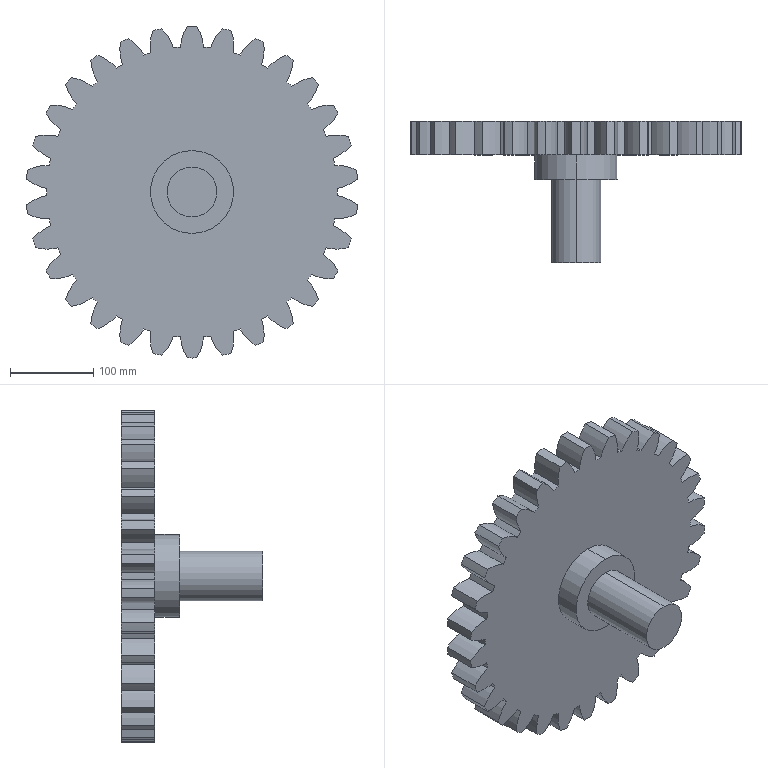Part | SolidWorks | features ICE 2, Extrusion 1 | 2 solids | 136 faces | box 398.808 x 170 x 400 mm | volume 5023065 mm3 | cylinder 131 | plane 5 | commonest cylinder face diameters 110 x66 400 x31 350 x30 60 x2 100 x2